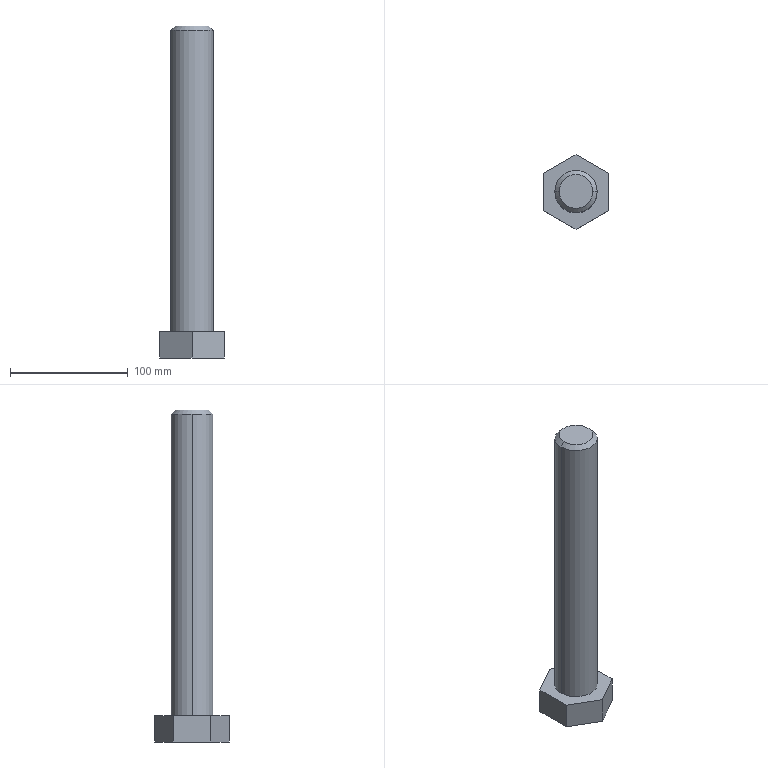Part | SolidWorks | features Chamfer 1, Extrusion 1, ICE 1, RefAxis 1 | 1 solid | 13 faces | box 55 x 63.509 x 282.5 mm | volume 322908 mm3 | plane 9 | cone 2 | cylinder 2 | commonest cylinder face diameters 36 x2
STEP:
#1=CARTESIAN_POINT('',(14.4,0.,282.5));
#2=VERTEX_POINT('',#1);
#3=CARTESIAN_POINT('',(-14.4,0.,282.5));
#4=VERTEX_POINT('',#3);
#5=CARTESIAN_POINT('',(0.,0.,282.5));
#6=DIRECTION('',(0.,0.,1.));
#7=DIRECTION('',(1.,0.,0.));
#8=AXIS2_PLACEMENT_3D('',#5,#6,#7);
#9=CIRCLE('',#8,14.4);
#10=EDGE_CURVE('',#2,#4,#9,.T.);
#11=ORIENTED_EDGE('',*,*,#10,.F.);
#12=CARTESIAN_POINT('',(18.,0.,278.9));
#13=VERTEX_POINT('',#12);
#14=CARTESIAN_POINT('',(14.4,0.,282.5));
#15=DIRECTION('',(0.7071,0.,-0.7071));
#16=VECTOR('',#15,1000.);
#17=LINE('',#14,#16);
#18=EDGE_CURVE('',#2,#13,#17,.T.);
#19=ORIENTED_EDGE('',*,*,#18,.T.);
#20=CARTESIAN_POINT('',(-18.,0.,278.9));
#21=VERTEX_POINT('',#20);
#22=CARTESIAN_POINT('',(0.,0.,278.9));
#23=DIRECTION('',(0.,0.,-1.));
#24=DIRECTION('',(1.,0.,0.));
#25=AXIS2_PLACEMENT_3D('',#22,#23,#24);
#26=CIRCLE('',#25,18.);
#27=EDGE_CURVE('',#21,#13,#26,.T.);
#28=ORIENTED_EDGE('',*,*,#27,.F.);
#29=CARTESIAN_POINT('',(-14.4,0.,282.5));
#30=DIRECTION('',(-0.7071,0.,-0.7071));
#31=VECTOR('',#30,1000.);
#32=LINE('',#29,#31);
#33=EDGE_CURVE('',#4,#21,#32,.T.);
#34=ORIENTED_EDGE('',*,*,#33,.F.);
#35=EDGE_LOOP('',(#11,#19,#28,#34));
#36=FACE_OUTER_BOUND('',#35,.T.);
#37=CARTESIAN_POINT('',(0.,0.,282.5));
#38=DIRECTION('',(0.,0.,-1.));
#39=DIRECTION('',(-1.,0.,0.));
#40=AXIS2_PLACEMENT_3D('',#37,#38,#39);
#41=CONICAL_SURFACE('',#40,14.4,0.7854);
#42=ADVANCED_FACE('',(#36),#41,.T.);
#43=ORIENTED_EDGE('',*,*,#27,.T.);
#44=CARTESIAN_POINT('',(18.,0.,22.5));
#45=VERTEX_POINT('',#44);
#46=CARTESIAN_POINT('',(18.,0.,282.5));
#47=DIRECTION('',(0.,0.,-1.));
#48=VECTOR('',#47,1000.);
#49=LINE('',#46,#48);
#50=EDGE_CURVE('',#13,#45,#49,.T.);
#51=ORIENTED_EDGE('',*,*,#50,.T.);
#52=CARTESIAN_POINT('',(-18.,0.,22.5));
#53=VERTEX_POINT('',#52);
#54=CARTESIAN_POINT('',(0.,0.,22.5));
#55=DIRECTION('',(0.,0.,1.));
#56=DIRECTION('',(1.,0.,0.));
#57=AXIS2_PLACEMENT_3D('',#54,#55,#56);
#58=CIRCLE('',#57,18.);
#59=EDGE_CURVE('',#45,#53,#58,.T.);
#60=ORIENTED_EDGE('',*,*,#59,.T.);
#61=CARTESIAN_POINT('',(-18.,0.,282.5));
#62=DIRECTION('',(0.,0.,-1.));
#63=VECTOR('',#62,1000.);
#64=LINE('',#61,#63);
#65=EDGE_CURVE('',#21,#53,#64,.T.);
#66=ORIENTED_EDGE('',*,*,#65,.F.);
#67=EDGE_LOOP('',(#43,#51,#60,#66));
#68=FACE_OUTER_BOUND('',#67,.T.);
#69=CARTESIAN_POINT('',(0.,0.,282.5));
#70=DIRECTION('',(0.,0.,-1.));
#71=DIRECTION('',(-1.,0.,0.));
#72=AXIS2_PLACEMENT_3D('',#69,#70,#71);
#73=CYLINDRICAL_SURFACE('',#72,18.);
#74=ADVANCED_FACE('',(#68),#73,.T.);
#75=CARTESIAN_POINT('',(27.5,-15.877,22.5));
#76=VERTEX_POINT('',#75);
#77=CARTESIAN_POINT('',(27.5,15.877,22.5));
#78=VERTEX_POINT('',#77);
#79=CARTESIAN_POINT('',(27.5,-15.877,22.5));
#80=DIRECTION('',(0.,1.,0.));
#81=VECTOR('',#80,1000.);
#82=LINE('',#79,#81);
#83=EDGE_CURVE('',#76,#78,#82,.T.);
#84=ORIENTED_EDGE('',*,*,#83,.T.);
#85=CARTESIAN_POINT('',(0.,31.754,22.5));
#86=VERTEX_POINT('',#85);
#87=CARTESIAN_POINT('',(27.5,15.877,22.5));
#88=DIRECTION('',(-0.866,0.5,0.));
#89=VECTOR('',#88,1000.);
#90=LINE('',#87,#89);
#91=EDGE_CURVE('',#78,#86,#90,.T.);
#92=ORIENTED_EDGE('',*,*,#91,.T.);
#93=CARTESIAN_POINT('',(-27.5,15.877,22.5));
#94=VERTEX_POINT('',#93);
#95=CARTESIAN_POINT('',(0.,31.754,22.5));
#96=DIRECTION('',(-0.866,-0.5,0.));
#97=VECTOR('',#96,1000.);
#98=LINE('',#95,#97);
#99=EDGE_CURVE('',#86,#94,#98,.T.);
#100=ORIENTED_EDGE('',*,*,#99,.T.);
#101=CARTESIAN_POINT('',(-27.5,-15.877,22.5));
#102=VERTEX_POINT('',#101);
#103=CARTESIAN_POINT('',(-27.5,15.877,22.5));
#104=DIRECTION('',(0.,-1.,0.));
#105=VECTOR('',#104,1000.);
#106=LINE('',#103,#105);
#107=EDGE_CURVE('',#94,#102,#106,.T.);
#108=ORIENTED_EDGE('',*,*,#107,.T.);
#109=CARTESIAN_POINT('',(0.,-31.754,22.5));
#110=VERTEX_POINT('',#109);
#111=CARTESIAN_POINT('',(-27.5,-15.877,22.5));
#112=DIRECTION('',(0.866,-0.5,0.));
#113=VECTOR('',#112,1000.);
#114=LINE('',#111,#113);
#115=EDGE_CURVE('',#102,#110,#114,.T.);
#116=ORIENTED_EDGE('',*,*,#115,.T.);
#117=CARTESIAN_POINT('',(0.,-31.754,22.5));
#118=DIRECTION('',(0.866,0.5,0.));
#119=VECTOR('',#118,1000.);
#120=LINE('',#117,#119);
#121=EDGE_CURVE('',#110,#76,#120,.T.);
#122=ORIENTED_EDGE('',*,*,#121,.T.);
#123=EDGE_LOOP('',(#84,#92,#100,#108,#116,#122));
#124=FACE_OUTER_BOUND('',#123,.T.);
#125=CARTESIAN_POINT('',(0.,0.,22.5));
#126=DIRECTION('',(0.,0.,1.));
#127=DIRECTION('',(1.,0.,0.));
#128=AXIS2_PLACEMENT_3D('',#125,#126,#127);
#129=CIRCLE('',#128,18.);
#130=EDGE_CURVE('',#53,#45,#129,.T.);
#131=ORIENTED_EDGE('',*,*,#130,.F.);
#132=ORIENTED_EDGE('',*,*,#59,.F.);
#133=EDGE_LOOP('',(#131,#132));
#134=FACE_BOUND('',#133,.T.);
#135=CARTESIAN_POINT('',(0.,0.,22.5));
#136=DIRECTION('',(0.,0.,1.));
#137=DIRECTION('',(1.,0.,0.));
#138=AXIS2_PLACEMENT_3D('',#135,#136,#137);
#139=PLANE('',#138);
#140=ADVANCED_FACE('',(#124,#134),#139,.T.);
#141=CARTESIAN_POINT('',(27.5,-15.877,0.));
#142=VERTEX_POINT('',#141);
#143=CARTESIAN_POINT('',(27.5,15.877,0.));
#144=VERTEX_POINT('',#143);
#145=CARTESIAN_POINT('',(27.5,-15.877,0.));
#146=DIRECTION('',(0.,1.,0.));
#147=VECTOR('',#146,1000.);
#148=LINE('',#145,#147);
#149=EDGE_CURVE('',#142,#144,#148,.T.);
#150=ORIENTED_EDGE('',*,*,#149,.T.);
#151=CARTESIAN_POINT('',(27.5,15.877,22.5));
#152=DIRECTION('',(0.,0.,-1.));
#153=VECTOR('',#152,1000.);
#154=LINE('',#151,#153);
#155=EDGE_CURVE('',#78,#144,#154,.T.);
#156=ORIENTED_EDGE('',*,*,#155,.F.);
#157=ORIENTED_EDGE('',*,*,#83,.F.);
#158=CARTESIAN_POINT('',(27.5,-15.877,22.5));
#159=DIRECTION('',(0.,0.,-1.));
#160=VECTOR('',#159,1000.);
#161=LINE('',#158,#160);
#162=EDGE_CURVE('',#76,#142,#161,.T.);
#163=ORIENTED_EDGE('',*,*,#162,.T.);
#164=EDGE_LOOP('',(#150,#156,#157,#163));
#165=FACE_OUTER_BOUND('',#164,.T.);
#166=CARTESIAN_POINT('',(27.5,-15.877,22.5));
#167=DIRECTION('',(-1.,0.,0.));
#168=DIRECTION('',(0.,-1.,0.));
#169=AXIS2_PLACEMENT_3D('',#166,#167,#168);
#170=PLANE('',#169);
#171=ADVANCED_FACE('',(#165),#170,.F.);
#172=CARTESIAN_POINT('',(0.,31.754,0.));
#173=VERTEX_POINT('',#172);
#174=CARTESIAN_POINT('',(27.5,15.877,0.));
#175=DIRECTION('',(-0.866,0.5,0.));
#176=VECTOR('',#175,1000.);
#177=LINE('',#174,#176);
#178=EDGE_CURVE('',#144,#173,#177,.T.);
#179=ORIENTED_EDGE('',*,*,#178,.T.);
#180=CARTESIAN_POINT('',(0.,31.754,22.5));
#181=DIRECTION('',(0.,0.,-1.));
#182=VECTOR('',#181,1000.);
#183=LINE('',#180,#182);
#184=EDGE_CURVE('',#86,#173,#183,.T.);
#185=ORIENTED_EDGE('',*,*,#184,.F.);
#186=ORIENTED_EDGE('',*,*,#91,.F.);
#187=ORIENTED_EDGE('',*,*,#155,.T.);
#188=EDGE_LOOP('',(#179,#185,#186,#187));
#189=FACE_OUTER_BOUND('',#188,.T.);
#190=CARTESIAN_POINT('',(27.5,15.877,22.5));
#191=DIRECTION('',(-0.5,-0.866,0.));
#192=DIRECTION('',(0.866,-0.5,0.));
#193=AXIS2_PLACEMENT_3D('',#190,#191,#192);
#194=PLANE('',#193);
#195=ADVANCED_FACE('',(#189),#194,.F.);
#196=CARTESIAN_POINT('',(-27.5,15.877,0.));
#197=VERTEX_POINT('',#196);
#198=CARTESIAN_POINT('',(0.,31.754,0.));
#199=DIRECTION('',(-0.866,-0.5,0.));
#200=VECTOR('',#199,1000.);
#201=LINE('',#198,#200);
#202=EDGE_CURVE('',#173,#197,#201,.T.);
#203=ORIENTED_EDGE('',*,*,#202,.T.);
#204=CARTESIAN_POINT('',(-27.5,15.877,22.5));
#205=DIRECTION('',(0.,0.,-1.));
#206=VECTOR('',#205,1000.);
#207=LINE('',#204,#206);
#208=EDGE_CURVE('',#94,#197,#207,.T.);
#209=ORIENTED_EDGE('',*,*,#208,.F.);
#210=ORIENTED_EDGE('',*,*,#99,.F.);
#211=ORIENTED_EDGE('',*,*,#184,.T.);
#212=EDGE_LOOP('',(#203,#209,#210,#211));
#213=FACE_OUTER_BOUND('',#212,.T.);
#214=CARTESIAN_POINT('',(0.,31.754,22.5));
#215=DIRECTION('',(0.5,-0.866,0.));
#216=DIRECTION('',(0.866,0.5,0.));
#217=AXIS2_PLACEMENT_3D('',#214,#215,#216);
#218=PLANE('',#217);
#219=ADVANCED_FACE('',(#213),#218,.F.);
#220=CARTESIAN_POINT('',(-27.5,-15.877,0.));
#221=VERTEX_POINT('',#220);
#222=CARTESIAN_POINT('',(-27.5,15.877,0.));
#223=DIRECTION('',(0.,-1.,0.));
#224=VECTOR('',#223,1000.);
#225=LINE('',#222,#224);
#226=EDGE_CURVE('',#197,#221,#225,.T.);
#227=ORIENTED_EDGE('',*,*,#226,.T.);
#228=CARTESIAN_POINT('',(-27.5,-15.877,22.5));
#229=DIRECTION('',(0.,0.,-1.));
#230=VECTOR('',#229,1000.);
#231=LINE('',#228,#230);
#232=EDGE_CURVE('',#102,#221,#231,.T.);
#233=ORIENTED_EDGE('',*,*,#232,.F.);
#234=ORIENTED_EDGE('',*,*,#107,.F.);
#235=ORIENTED_EDGE('',*,*,#208,.T.);
#236=EDGE_LOOP('',(#227,#233,#234,#235));
#237=FACE_OUTER_BOUND('',#236,.T.);
#238=CARTESIAN_POINT('',(-27.5,15.877,22.5));
#239=DIRECTION('',(1.,0.,0.));
#240=DIRECTION('',(0.,1.,0.));
#241=AXIS2_PLACEMENT_3D('',#238,#239,#240);
#242=PLANE('',#241);
#243=ADVANCED_FACE('',(#237),#242,.F.);
#244=CARTESIAN_POINT('',(0.,-31.754,0.));
#245=VERTEX_POINT('',#244);
#246=CARTESIAN_POINT('',(-27.5,-15.877,0.));
#247=DIRECTION('',(0.866,-0.5,0.));
#248=VECTOR('',#247,1000.);
#249=LINE('',#246,#248);
#250=EDGE_CURVE('',#221,#245,#249,.T.);
#251=ORIENTED_EDGE('',*,*,#250,.T.);
#252=CARTESIAN_POINT('',(0.,-31.754,22.5));
#253=DIRECTION('',(0.,0.,-1.));
#254=VECTOR('',#253,1000.);
#255=LINE('',#252,#254);
#256=EDGE_CURVE('',#110,#245,#255,.T.);
#257=ORIENTED_EDGE('',*,*,#256,.F.);
#258=ORIENTED_EDGE('',*,*,#115,.F.);
#259=ORIENTED_EDGE('',*,*,#232,.T.);
#260=EDGE_LOOP('',(#251,#257,#258,#259));
#261=FACE_OUTER_BOUND('',#260,.T.);
#262=CARTESIAN_POINT('',(-27.5,-15.877,22.5));
#263=DIRECTION('',(0.5,0.866,0.));
#264=DIRECTION('',(-0.866,0.5,0.));
#265=AXIS2_PLACEMENT_3D('',#262,#263,#264);
#266=PLANE('',#265);
#267=ADVANCED_FACE('',(#261),#266,.F.);
#268=CARTESIAN_POINT('',(0.,-31.754,0.));
#269=DIRECTION('',(0.866,0.5,0.));
#270=VECTOR('',#269,1000.);
#271=LINE('',#268,#270);
#272=EDGE_CURVE('',#245,#142,#271,.T.);
#273=ORIENTED_EDGE('',*,*,#272,.T.);
#274=ORIENTED_EDGE('',*,*,#162,.F.);
#275=ORIENTED_EDGE('',*,*,#121,.F.);
#276=ORIENTED_EDGE('',*,*,#256,.T.);
#277=EDGE_LOOP('',(#273,#274,#275,#276));
#278=FACE_OUTER_BOUND('',#277,.T.);
#279=CARTESIAN_POINT('',(0.,-31.754,22.5));
#280=DIRECTION('',(-0.5,0.866,0.));
#281=DIRECTION('',(-0.866,-0.5,0.));
#282=AXIS2_PLACEMENT_3D('',#279,#280,#281);
#283=PLANE('',#282);
#284=ADVANCED_FACE('',(#278),#283,.F.);
#285=ORIENTED_EDGE('',*,*,#149,.F.);
#286=ORIENTED_EDGE('',*,*,#272,.F.);
#287=ORIENTED_EDGE('',*,*,#250,.F.);
#288=ORIENTED_EDGE('',*,*,#226,.F.);
#289=ORIENTED_EDGE('',*,*,#202,.F.);
#290=ORIENTED_EDGE('',*,*,#178,.F.);
#291=EDGE_LOOP('',(#285,#286,#287,#288,#289,#290));
#292=FACE_OUTER_BOUND('',#291,.T.);
#293=CARTESIAN_POINT('',(0.,0.,0.));
#294=DIRECTION('',(0.,0.,1.));
#295=DIRECTION('',(1.,0.,0.));
#296=AXIS2_PLACEMENT_3D('',#293,#294,#295);
#297=PLANE('',#296);
#298=ADVANCED_FACE('',(#292),#297,.F.);
#299=ORIENTED_EDGE('',*,*,#50,.F.);
#300=CARTESIAN_POINT('',(0.,0.,278.9));
#301=DIRECTION('',(0.,0.,-1.));
#302=DIRECTION('',(1.,0.,0.));
#303=AXIS2_PLACEMENT_3D('',#300,#301,#302);
#304=CIRCLE('',#303,18.);
#305=EDGE_CURVE('',#13,#21,#304,.T.);
#306=ORIENTED_EDGE('',*,*,#305,.T.);
#307=ORIENTED_EDGE('',*,*,#65,.T.);
#308=ORIENTED_EDGE('',*,*,#130,.T.);
#309=EDGE_LOOP('',(#299,#306,#307,#308));
#310=FACE_OUTER_BOUND('',#309,.T.);
#311=CARTESIAN_POINT('',(0.,0.,282.5));
#312=DIRECTION('',(0.,0.,-1.));
#313=DIRECTION('',(-1.,0.,0.));
#314=AXIS2_PLACEMENT_3D('',#311,#312,#313);
#315=CYLINDRICAL_SURFACE('',#314,18.);
#316=ADVANCED_FACE('',(#310),#315,.T.);
#317=CARTESIAN_POINT('',(0.,0.,282.5));
#318=DIRECTION('',(0.,0.,1.));
#319=DIRECTION('',(1.,0.,0.));
#320=AXIS2_PLACEMENT_3D('',#317,#318,#319);
#321=CIRCLE('',#320,14.4);
#322=EDGE_CURVE('',#4,#2,#321,.T.);
#323=ORIENTED_EDGE('',*,*,#322,.T.);
#324=ORIENTED_EDGE('',*,*,#10,.T.);
#325=EDGE_LOOP('',(#323,#324));
#326=FACE_OUTER_BOUND('',#325,.T.);
#327=CARTESIAN_POINT('',(0.,0.,282.5));
#328=DIRECTION('',(0.,0.,1.));
#329=DIRECTION('',(1.,0.,0.));
#330=AXIS2_PLACEMENT_3D('',#327,#328,#329);
#331=PLANE('',#330);
#332=ADVANCED_FACE('',(#326),#331,.T.);
#333=ORIENTED_EDGE('',*,*,#18,.F.);
#334=ORIENTED_EDGE('',*,*,#322,.F.);
#335=ORIENTED_EDGE('',*,*,#33,.T.);
#336=ORIENTED_EDGE('',*,*,#305,.F.);
#337=EDGE_LOOP('',(#333,#334,#335,#336));
#338=FACE_OUTER_BOUND('',#337,.T.);
#339=CARTESIAN_POINT('',(0.,0.,282.5));
#340=DIRECTION('',(0.,0.,-1.));
#341=DIRECTION('',(-1.,0.,0.));
#342=AXIS2_PLACEMENT_3D('',#339,#340,#341);
#343=CONICAL_SURFACE('',#342,14.4,0.7854);
#344=ADVANCED_FACE('',(#338),#343,.T.);
#345=CLOSED_SHELL('',(#42,#74,#140,#171,#195,#219,#243,#267,#284,#298,#316,#332,#344));
#346=MANIFOLD_SOLID_BREP('',#345);
#347=CARTESIAN_POINT('',(0.,0.,0.));
#348=DIRECTION('',(0.,0.,1.));
#349=DIRECTION('',(1.,0.,0.));
#350=AXIS2_PLACEMENT_3D('',#347,#348,#349);
#351=(LENGTH_UNIT()NAMED_UNIT(*)SI_UNIT(.MILLI.,.METRE.));
#352=UNCERTAINTY_MEASURE_WITH_UNIT(LENGTH_MEASURE(0.00001),#351,'','');
#353=(NAMED_UNIT(*)PLANE_ANGLE_UNIT()SI_UNIT($,.RADIAN.));
#354=(NAMED_UNIT(*)SI_UNIT($,.STERADIAN.)SOLID_ANGLE_UNIT());
#355=(GEOMETRIC_REPRESENTATION_CONTEXT(3)GLOBAL_UNCERTAINTY_ASSIGNED_CONTEXT((#352))GLOBAL_UNIT_ASSIGNED_CONTEXT((#351,#353,#354))REPRESENTATION_CONTEXT('',''));
#356=ADVANCED_BREP_SHAPE_REPRESENTATION('',(#346,#350),#355);